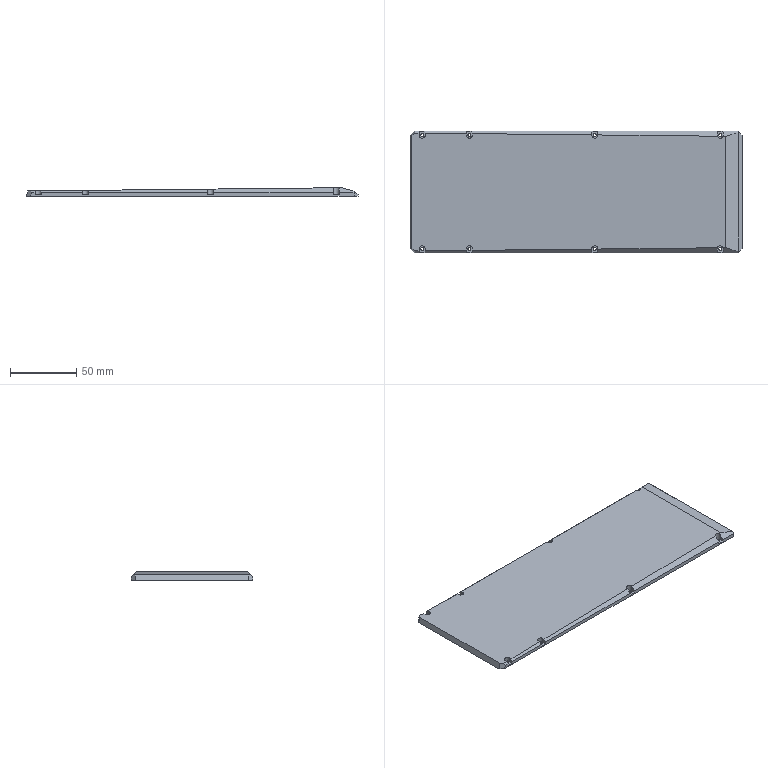NC program | NX | posted with a generic post | part box 251.5 x 92 x 6.5 mm
Whole program:
N10 G17 G21 G94 G90
(FLOOR_FACING , TOOL : D12-36-D12-120-3TFINISH)
N12 T01 M6
N14 G54
N16 G17 G0 G90 X3.9 Y63.385 S4000 M3
N18 G43 Z30. H1
N20 Z1.
N22 G94 G1 Y83.65 Z0.646 F2000.
N24 X-3.9 Z0.51
N26 Y0. Z-0.95
N28 Y-83.65
N30 X3.9
N32 Y83.65
N34 X-3.9
N36 Y0.
N38 X-12.9
N40 Y-92.65
N42 X12.9
N44 Y92.65
N46 X-12.9
N48 Y0.
N50 X-21.9
N52 Y-101.65
N54 X21.9
N56 Y101.65
N58 X-21.9
N60 Y0.
N62 X-30.9
N64 Y-110.65
N66 X30.9
N68 Y110.65
N70 X-30.9
N72 Y0.
N74 X-39.9
N76 Y-119.65
N78 X39.9
N80 Y119.65
N82 X-39.9
N84 Y0.
N86 Y-1.
N88 Z0.05
N90 G0 Z30.
N92 X3.9 Y63.385
N94 Z0.05
N96 G1 Y83.65 Z-0.304
N98 X-3.9 Z-0.44
N100 Y0. Z-1.9
N102 Y-83.65
N104 X3.9
N106 Y83.65
N108 X-3.9
N110 Y0.
N112 X-12.9
N114 Y-92.65
N116 X12.9
N118 Y92.65
N120 X-12.9
N122 Y0.
N124 X-21.9
N126 Y-101.65
N128 X21.9
N130 Y101.65
N132 X-21.9
N134 Y0.
N136 X-30.9
N138 Y-110.65
N140 X30.9
N142 Y110.65
N144 X-30.9
N146 Y0.
N148 X-39.9
N150 Y-119.65
N152 X39.9
N154 Y119.65
N156 X-39.9
N158 Y0.
N160 Y-1.
N162 Z-0.9
N164 G0 Z30.
N166 M5
N168 M2